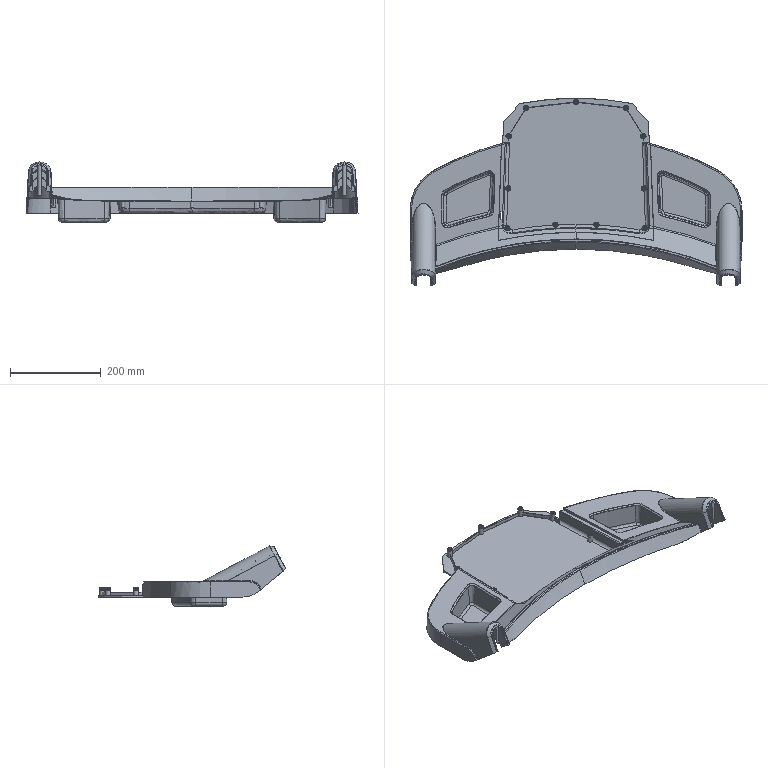Part | STEP file | 5091204W | 1 solid | 722 faces | box 729.86 x 412.544 x 132.193 mm | volume 994428 mm3 | plane 269 | spline 202 | cylinder 152 | cone 99 | commonest cylinder face diameters 4 x25 3 x14 6 x14 44 x14 10 x12 3.5 x11